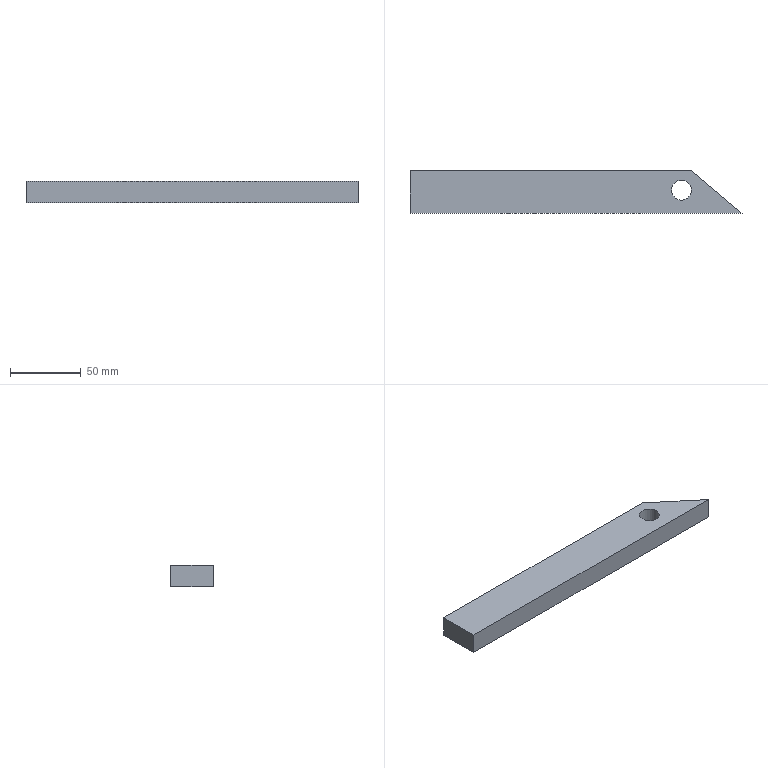Part | NX | features solid 2 | 1 solid | 7 faces | box 234.258 x 30 x 15 mm | volume 95063 mm3 | plane 6 | cylinder 1 | commonest cylinder face diameters 14 x1
STEP:
#1=CARTESIAN_POINT('',(-430.,-95.,15.));
#2=VERTEX_POINT('',#1);
#3=CARTESIAN_POINT('',(-195.742,-95.,15.));
#4=VERTEX_POINT('',#3);
#5=CARTESIAN_POINT('',(-410.,-95.,15.));
#6=DIRECTION('',(-1.,0.,0.));
#7=VECTOR('',#6,1000.);
#8=LINE('',#5,#7);
#9=EDGE_CURVE('',#2,#4,#8,.F.);
#10=ORIENTED_EDGE('',*,*,#9,.T.);
#11=CARTESIAN_POINT('',(-231.495,-65.,15.));
#12=VERTEX_POINT('',#11);
#13=CARTESIAN_POINT('',(-336.246,22.897,15.));
#14=DIRECTION('',(-0.766,0.6428,0.));
#15=VECTOR('',#14,1000.);
#16=LINE('',#13,#15);
#17=EDGE_CURVE('',#12,#4,#16,.F.);
#18=ORIENTED_EDGE('',*,*,#17,.F.);
#19=CARTESIAN_POINT('',(-430.,-65.,15.));
#20=VERTEX_POINT('',#19);
#21=CARTESIAN_POINT('',(-410.,-65.,15.));
#22=DIRECTION('',(-1.,0.,0.));
#23=VECTOR('',#22,1000.);
#24=LINE('',#21,#23);
#25=EDGE_CURVE('',#20,#12,#24,.F.);
#26=ORIENTED_EDGE('',*,*,#25,.F.);
#27=CARTESIAN_POINT('',(-430.,-65.,15.));
#28=DIRECTION('',(0.,1.,0.));
#29=VECTOR('',#28,1000.);
#30=LINE('',#27,#29);
#31=EDGE_CURVE('',#20,#2,#30,.F.);
#32=ORIENTED_EDGE('',*,*,#31,.T.);
#33=EDGE_LOOP('',(#10,#18,#26,#32));
#34=FACE_BOUND('',#33,.T.);
#35=CARTESIAN_POINT('',(-245.471,-78.728,15.));
#36=VERTEX_POINT('',#35);
#37=CARTESIAN_POINT('',(-238.471,-78.728,15.));
#38=DIRECTION('',(0.,0.,-1.));
#39=DIRECTION('',(-1.,0.,0.));
#40=AXIS2_PLACEMENT_3D('',#37,#38,#39);
#41=CIRCLE('',#40,7.);
#42=EDGE_CURVE('',#36,#36,#41,.F.);
#43=ORIENTED_EDGE('',*,*,#42,.F.);
#44=EDGE_LOOP('',(#43));
#45=FACE_BOUND('',#44,.T.);
#46=CARTESIAN_POINT('',(-410.,-65.,15.));
#47=DIRECTION('',(0.,0.,-1.));
#48=DIRECTION('',(-1.,0.,0.));
#49=AXIS2_PLACEMENT_3D('',#46,#47,#48);
#50=PLANE('',#49);
#51=ADVANCED_FACE('',(#34,#45),#50,.F.);
#52=CARTESIAN_POINT('',(-430.,-95.,0.));
#53=VERTEX_POINT('',#52);
#54=CARTESIAN_POINT('',(-195.742,-95.,0.));
#55=VERTEX_POINT('',#54);
#56=CARTESIAN_POINT('',(-410.,-95.,0.));
#57=DIRECTION('',(1.,0.,0.));
#58=VECTOR('',#57,1000.);
#59=LINE('',#56,#58);
#60=EDGE_CURVE('',#53,#55,#59,.T.);
#61=ORIENTED_EDGE('',*,*,#60,.F.);
#62=CARTESIAN_POINT('',(-430.,-65.,0.));
#63=VERTEX_POINT('',#62);
#64=CARTESIAN_POINT('',(-430.,-65.,0.));
#65=DIRECTION('',(0.,1.,0.));
#66=VECTOR('',#65,1000.);
#67=LINE('',#64,#66);
#68=EDGE_CURVE('',#63,#53,#67,.F.);
#69=ORIENTED_EDGE('',*,*,#68,.F.);
#70=CARTESIAN_POINT('',(-231.495,-65.,0.));
#71=VERTEX_POINT('',#70);
#72=CARTESIAN_POINT('',(-410.,-65.,0.));
#73=DIRECTION('',(1.,0.,0.));
#74=VECTOR('',#73,1000.);
#75=LINE('',#72,#74);
#76=EDGE_CURVE('',#63,#71,#75,.T.);
#77=ORIENTED_EDGE('',*,*,#76,.T.);
#78=CARTESIAN_POINT('',(-336.246,22.897,0.));
#79=DIRECTION('',(-0.766,0.6428,0.));
#80=VECTOR('',#79,1000.);
#81=LINE('',#78,#80);
#82=EDGE_CURVE('',#71,#55,#81,.F.);
#83=ORIENTED_EDGE('',*,*,#82,.T.);
#84=EDGE_LOOP('',(#61,#69,#77,#83));
#85=FACE_BOUND('',#84,.T.);
#86=CARTESIAN_POINT('',(-245.471,-78.728,0.));
#87=VERTEX_POINT('',#86);
#88=CARTESIAN_POINT('',(-238.471,-78.728,0.));
#89=DIRECTION('',(0.,0.,-1.));
#90=DIRECTION('',(-1.,0.,0.));
#91=AXIS2_PLACEMENT_3D('',#88,#89,#90);
#92=CIRCLE('',#91,7.);
#93=EDGE_CURVE('',#87,#87,#92,.F.);
#94=ORIENTED_EDGE('',*,*,#93,.T.);
#95=EDGE_LOOP('',(#94));
#96=FACE_BOUND('',#95,.T.);
#97=CARTESIAN_POINT('',(-410.,-65.,0.));
#98=DIRECTION('',(0.,0.,-1.));
#99=DIRECTION('',(-1.,0.,0.));
#100=AXIS2_PLACEMENT_3D('',#97,#98,#99);
#101=PLANE('',#100);
#102=ADVANCED_FACE('',(#85,#96),#101,.T.);
#103=CARTESIAN_POINT('',(-231.495,-65.,-15.));
#104=DIRECTION('',(0.,0.,-1.));
#105=VECTOR('',#104,1000.);
#106=LINE('',#103,#105);
#107=EDGE_CURVE('',#71,#12,#106,.F.);
#108=ORIENTED_EDGE('',*,*,#107,.F.);
#109=ORIENTED_EDGE('',*,*,#76,.F.);
#110=CARTESIAN_POINT('',(-430.,-65.,0.));
#111=DIRECTION('',(0.,0.,-1.));
#112=VECTOR('',#111,1000.);
#113=LINE('',#110,#112);
#114=EDGE_CURVE('',#63,#20,#113,.F.);
#115=ORIENTED_EDGE('',*,*,#114,.T.);
#116=ORIENTED_EDGE('',*,*,#25,.T.);
#117=EDGE_LOOP('',(#108,#109,#115,#116));
#118=FACE_BOUND('',#117,.T.);
#119=CARTESIAN_POINT('',(-410.,-65.,0.));
#120=DIRECTION('',(0.,1.,0.));
#121=DIRECTION('',(1.,0.,0.));
#122=AXIS2_PLACEMENT_3D('',#119,#120,#121);
#123=PLANE('',#122);
#124=ADVANCED_FACE('',(#118),#123,.T.);
#125=ORIENTED_EDGE('',*,*,#114,.F.);
#126=ORIENTED_EDGE('',*,*,#68,.T.);
#127=CARTESIAN_POINT('',(-430.,-95.,0.));
#128=DIRECTION('',(0.,0.,1.));
#129=VECTOR('',#128,1000.);
#130=LINE('',#127,#129);
#131=EDGE_CURVE('',#53,#2,#130,.T.);
#132=ORIENTED_EDGE('',*,*,#131,.T.);
#133=ORIENTED_EDGE('',*,*,#31,.F.);
#134=EDGE_LOOP('',(#125,#126,#132,#133));
#135=FACE_BOUND('',#134,.T.);
#136=CARTESIAN_POINT('',(-430.,-65.,0.));
#137=DIRECTION('',(1.,0.,0.));
#138=DIRECTION('',(0.,-1.,0.));
#139=AXIS2_PLACEMENT_3D('',#136,#137,#138);
#140=PLANE('',#139);
#141=ADVANCED_FACE('',(#135),#140,.F.);
#142=ORIENTED_EDGE('',*,*,#131,.F.);
#143=ORIENTED_EDGE('',*,*,#60,.T.);
#144=CARTESIAN_POINT('',(-195.742,-95.,0.));
#145=DIRECTION('',(0.,0.,1.));
#146=VECTOR('',#145,1000.);
#147=LINE('',#144,#146);
#148=EDGE_CURVE('',#55,#4,#147,.T.);
#149=ORIENTED_EDGE('',*,*,#148,.T.);
#150=ORIENTED_EDGE('',*,*,#9,.F.);
#151=EDGE_LOOP('',(#142,#143,#149,#150));
#152=FACE_BOUND('',#151,.T.);
#153=CARTESIAN_POINT('',(-410.,-95.,0.));
#154=DIRECTION('',(0.,1.,0.));
#155=DIRECTION('',(1.,0.,0.));
#156=AXIS2_PLACEMENT_3D('',#153,#154,#155);
#157=PLANE('',#156);
#158=ADVANCED_FACE('',(#152),#157,.F.);
#159=ORIENTED_EDGE('',*,*,#82,.F.);
#160=ORIENTED_EDGE('',*,*,#107,.T.);
#161=ORIENTED_EDGE('',*,*,#17,.T.);
#162=ORIENTED_EDGE('',*,*,#148,.F.);
#163=EDGE_LOOP('',(#159,#160,#161,#162));
#164=FACE_BOUND('',#163,.T.);
#165=CARTESIAN_POINT('',(-274.791,-28.67,-15.));
#166=DIRECTION('',(-0.6428,-0.766,0.));
#167=DIRECTION('',(0.766,-0.6428,0.));
#168=AXIS2_PLACEMENT_3D('',#165,#166,#167);
#169=PLANE('',#168);
#170=ADVANCED_FACE('',(#164),#169,.F.);
#171=ORIENTED_EDGE('',*,*,#93,.F.);
#172=EDGE_LOOP('',(#171));
#173=FACE_BOUND('',#172,.T.);
#174=ORIENTED_EDGE('',*,*,#42,.T.);
#175=EDGE_LOOP('',(#174));
#176=FACE_BOUND('',#175,.T.);
#177=CARTESIAN_POINT('',(-238.471,-78.728,-200.));
#178=DIRECTION('',(0.,0.,1.));
#179=DIRECTION('',(1.,0.,0.));
#180=AXIS2_PLACEMENT_3D('',#177,#178,#179);
#181=CYLINDRICAL_SURFACE('',#180,7.);
#182=ADVANCED_FACE('',(#173,#176),#181,.F.);
#183=CLOSED_SHELL('',(#51,#102,#124,#141,#158,#170,#182));
#184=MANIFOLD_SOLID_BREP('',#183);
#185=(LENGTH_UNIT()NAMED_UNIT(*)SI_UNIT(.MILLI.,.METRE.));
#186=UNCERTAINTY_MEASURE_WITH_UNIT(LENGTH_MEASURE(0.00001),#185,'','');
#187=(NAMED_UNIT(*)PLANE_ANGLE_UNIT()SI_UNIT($,.RADIAN.));
#188=(NAMED_UNIT(*)SI_UNIT($,.STERADIAN.)SOLID_ANGLE_UNIT());
#189=(GEOMETRIC_REPRESENTATION_CONTEXT(3)GLOBAL_UNCERTAINTY_ASSIGNED_CONTEXT((#186))GLOBAL_UNIT_ASSIGNED_CONTEXT((#185,#187,#188))REPRESENTATION_CONTEXT('',''));
#190=ADVANCED_BREP_SHAPE_REPRESENTATION('',(#184),#189);